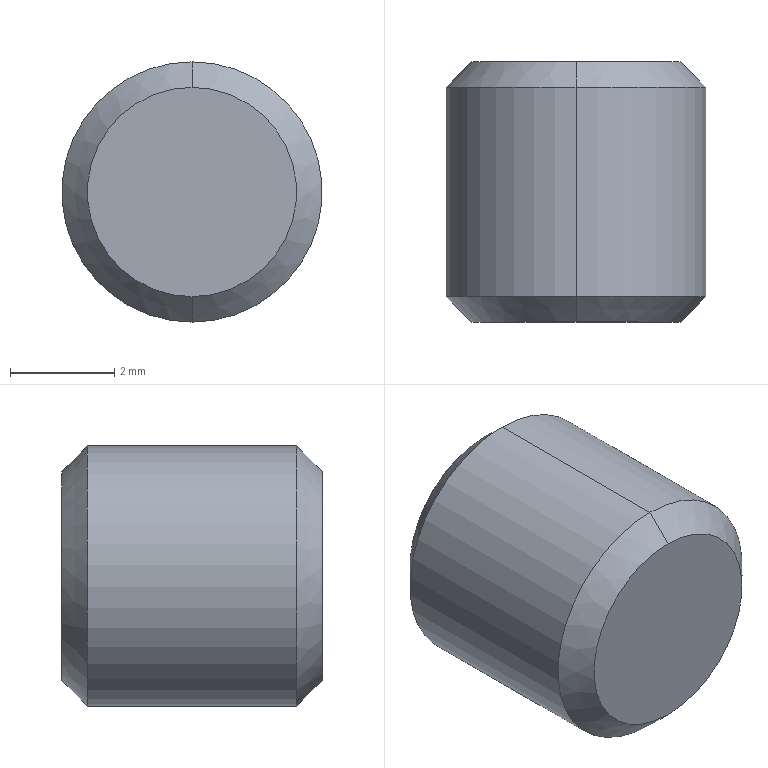Part | STEP file | 2-2 | 1 solid | 15 faces | box 5 x 5 x 5 mm | volume 86.524 mm3 | plane 9 | cone 4 | cylinder 2 | commonest cylinder face diameters 5 x2
STEP:
#1=CARTESIAN_POINT('',(0.,0.,0.));
#2=DIRECTION('',(0.,0.,1.));
#3=DIRECTION('',(1.,0.,0.));
#4=AXIS2_PLACEMENT_3D('',#1,#2,#3);
#5=CARTESIAN_POINT('',(10.278,45.,1.25));
#6=VERTEX_POINT('',#5);
#7=CARTESIAN_POINT('',(11.722,45.,1.25));
#8=VERTEX_POINT('',#7);
#9=CARTESIAN_POINT('',(10.278,45.,1.25));
#10=DIRECTION('',(1.,0.,0.));
#11=VECTOR('',#10,1.);
#12=LINE('',#9,#11);
#13=CARTESIAN_POINT('',(11.,45.,0.));
#14=DIRECTION('',(0.,1.,0.));
#15=DIRECTION('',(0.,0.,-1.));
#16=AXIS2_PLACEMENT_3D('',#13,#14,#15);
#17=PLANE('',#16);
#18=CARTESIAN_POINT('',(-1.25,0.7217));
#19=DIRECTION('',(0.,-1.));
#20=VECTOR('',#19,1.);
#21=LINE('',#18,#20);
#22=(GEOMETRIC_REPRESENTATION_CONTEXT(2)PARAMETRIC_REPRESENTATION_CONTEXT()REPRESENTATION_CONTEXT('',''));
#23=DEFINITIONAL_REPRESENTATION('',(#21),#22);
#24=PCURVE('',#17,#23);
#25=CARTESIAN_POINT('',(10.278,46.5,1.25));
#26=DIRECTION('',(0.,0.,1.));
#27=DIRECTION('',(1.,0.,0.));
#28=AXIS2_PLACEMENT_3D('',#25,#26,#27);
#29=PLANE('',#28);
#30=CARTESIAN_POINT('',(0.,-1.5));
#31=DIRECTION('',(1.,0.));
#32=VECTOR('',#31,1.);
#33=LINE('',#30,#32);
#34=(GEOMETRIC_REPRESENTATION_CONTEXT(2)PARAMETRIC_REPRESENTATION_CONTEXT()REPRESENTATION_CONTEXT('',''));
#35=DEFINITIONAL_REPRESENTATION('',(#33),#34);
#36=PCURVE('',#29,#35);
#37=SURFACE_CURVE('',#12,(#24,#36),.PCURVE_S1.);
#38=EDGE_CURVE('',#6,#8,#37,.T.);
#39=ORIENTED_EDGE('',*,*,#38,.T.);
#40=CARTESIAN_POINT('',(12.443,45.,0.));
#41=VERTEX_POINT('',#40);
#42=CARTESIAN_POINT('',(11.722,45.,1.25));
#43=DIRECTION('',(0.5,0.,-0.866));
#44=VECTOR('',#43,1.);
#45=LINE('',#42,#44);
#46=CARTESIAN_POINT('',(-1.25,-0.7217));
#47=DIRECTION('',(0.866,-0.5));
#48=VECTOR('',#47,1.);
#49=LINE('',#46,#48);
#50=(GEOMETRIC_REPRESENTATION_CONTEXT(2)PARAMETRIC_REPRESENTATION_CONTEXT()REPRESENTATION_CONTEXT('',''));
#51=DEFINITIONAL_REPRESENTATION('',(#49),#50);
#52=PCURVE('',#17,#51);
#53=CARTESIAN_POINT('',(11.722,46.5,1.25));
#54=DIRECTION('',(0.866,0.,0.5));
#55=DIRECTION('',(0.,-1.,0.));
#56=AXIS2_PLACEMENT_3D('',#53,#54,#55);
#57=PLANE('',#56);
#58=CARTESIAN_POINT('',(1.5,0.));
#59=DIRECTION('',(0.,1.));
#60=VECTOR('',#59,1.);
#61=LINE('',#58,#60);
#62=(GEOMETRIC_REPRESENTATION_CONTEXT(2)PARAMETRIC_REPRESENTATION_CONTEXT()REPRESENTATION_CONTEXT('',''));
#63=DEFINITIONAL_REPRESENTATION('',(#61),#62);
#64=PCURVE('',#57,#63);
#65=SURFACE_CURVE('',#45,(#52,#64),.PCURVE_S1.);
#66=EDGE_CURVE('',#8,#41,#65,.T.);
#67=ORIENTED_EDGE('',*,*,#66,.T.);
#68=CARTESIAN_POINT('',(11.722,45.,-1.25));
#69=VERTEX_POINT('',#68);
#70=CARTESIAN_POINT('',(12.443,45.,0.));
#71=DIRECTION('',(-0.5,0.,-0.866));
#72=VECTOR('',#71,1.);
#73=LINE('',#70,#72);
#74=CARTESIAN_POINT('',(0.,-1.443));
#75=DIRECTION('',(0.866,0.5));
#76=VECTOR('',#75,1.);
#77=LINE('',#74,#76);
#78=(GEOMETRIC_REPRESENTATION_CONTEXT(2)PARAMETRIC_REPRESENTATION_CONTEXT()REPRESENTATION_CONTEXT('',''));
#79=DEFINITIONAL_REPRESENTATION('',(#77),#78);
#80=PCURVE('',#17,#79);
#81=CARTESIAN_POINT('',(12.443,46.5,0.));
#82=DIRECTION('',(0.866,0.,-0.5));
#83=DIRECTION('',(0.,-1.,0.));
#84=AXIS2_PLACEMENT_3D('',#81,#82,#83);
#85=PLANE('',#84);
#86=CARTESIAN_POINT('',(1.5,0.));
#87=DIRECTION('',(0.,1.));
#88=VECTOR('',#87,1.);
#89=LINE('',#86,#88);
#90=(GEOMETRIC_REPRESENTATION_CONTEXT(2)PARAMETRIC_REPRESENTATION_CONTEXT()REPRESENTATION_CONTEXT('',''));
#91=DEFINITIONAL_REPRESENTATION('',(#89),#90);
#92=PCURVE('',#85,#91);
#93=SURFACE_CURVE('',#73,(#80,#92),.PCURVE_S1.);
#94=EDGE_CURVE('',#41,#69,#93,.T.);
#95=ORIENTED_EDGE('',*,*,#94,.T.);
#96=CARTESIAN_POINT('',(10.278,45.,-1.25));
#97=VERTEX_POINT('',#96);
#98=CARTESIAN_POINT('',(11.722,45.,-1.25));
#99=DIRECTION('',(-1.,0.,0.));
#100=VECTOR('',#99,1.);
#101=LINE('',#98,#100);
#102=CARTESIAN_POINT('',(1.25,-0.7217));
#103=DIRECTION('',(0.,1.));
#104=VECTOR('',#103,1.);
#105=LINE('',#102,#104);
#106=(GEOMETRIC_REPRESENTATION_CONTEXT(2)PARAMETRIC_REPRESENTATION_CONTEXT()REPRESENTATION_CONTEXT('',''));
#107=DEFINITIONAL_REPRESENTATION('',(#105),#106);
#108=PCURVE('',#17,#107);
#109=CARTESIAN_POINT('',(11.722,46.5,-1.25));
#110=DIRECTION('',(0.,0.,-1.));
#111=DIRECTION('',(-1.,0.,0.));
#112=AXIS2_PLACEMENT_3D('',#109,#110,#111);
#113=PLANE('',#112);
#114=CARTESIAN_POINT('',(0.,-1.5));
#115=DIRECTION('',(1.,0.));
#116=VECTOR('',#115,1.);
#117=LINE('',#114,#116);
#118=(GEOMETRIC_REPRESENTATION_CONTEXT(2)PARAMETRIC_REPRESENTATION_CONTEXT()REPRESENTATION_CONTEXT('',''));
#119=DEFINITIONAL_REPRESENTATION('',(#117),#118);
#120=PCURVE('',#113,#119);
#121=SURFACE_CURVE('',#101,(#108,#120),.PCURVE_S1.);
#122=EDGE_CURVE('',#69,#97,#121,.T.);
#123=ORIENTED_EDGE('',*,*,#122,.T.);
#124=CARTESIAN_POINT('',(9.557,45.,0.));
#125=VERTEX_POINT('',#124);
#126=CARTESIAN_POINT('',(10.278,45.,-1.25));
#127=DIRECTION('',(-0.5,0.,0.866));
#128=VECTOR('',#127,1.);
#129=LINE('',#126,#128);
#130=CARTESIAN_POINT('',(1.25,0.7217));
#131=DIRECTION('',(-0.866,0.5));
#132=VECTOR('',#131,1.);
#133=LINE('',#130,#132);
#134=(GEOMETRIC_REPRESENTATION_CONTEXT(2)PARAMETRIC_REPRESENTATION_CONTEXT()REPRESENTATION_CONTEXT('',''));
#135=DEFINITIONAL_REPRESENTATION('',(#133),#134);
#136=PCURVE('',#17,#135);
#137=CARTESIAN_POINT('',(10.278,46.5,-1.25));
#138=DIRECTION('',(-0.866,0.,-0.5));
#139=DIRECTION('',(-0.5,0.,0.866));
#140=AXIS2_PLACEMENT_3D('',#137,#138,#139);
#141=PLANE('',#140);
#142=CARTESIAN_POINT('',(0.,-1.5));
#143=DIRECTION('',(1.,0.));
#144=VECTOR('',#143,1.);
#145=LINE('',#142,#144);
#146=(GEOMETRIC_REPRESENTATION_CONTEXT(2)PARAMETRIC_REPRESENTATION_CONTEXT()REPRESENTATION_CONTEXT('',''));
#147=DEFINITIONAL_REPRESENTATION('',(#145),#146);
#148=PCURVE('',#141,#147);
#149=SURFACE_CURVE('',#129,(#136,#148),.PCURVE_S1.);
#150=EDGE_CURVE('',#97,#125,#149,.T.);
#151=ORIENTED_EDGE('',*,*,#150,.T.);
#152=CARTESIAN_POINT('',(9.557,45.,0.));
#153=DIRECTION('',(0.5,0.,0.866));
#154=VECTOR('',#153,1.);
#155=LINE('',#152,#154);
#156=CARTESIAN_POINT('',(0.,1.443));
#157=DIRECTION('',(-0.866,-0.5));
#158=VECTOR('',#157,1.);
#159=LINE('',#156,#158);
#160=(GEOMETRIC_REPRESENTATION_CONTEXT(2)PARAMETRIC_REPRESENTATION_CONTEXT()REPRESENTATION_CONTEXT('',''));
#161=DEFINITIONAL_REPRESENTATION('',(#159),#160);
#162=PCURVE('',#17,#161);
#163=CARTESIAN_POINT('',(9.557,46.5,0.));
#164=DIRECTION('',(-0.866,0.,0.5));
#165=DIRECTION('',(0.,1.,0.));
#166=AXIS2_PLACEMENT_3D('',#163,#164,#165);
#167=PLANE('',#166);
#168=CARTESIAN_POINT('',(-1.5,0.));
#169=DIRECTION('',(0.,-1.));
#170=VECTOR('',#169,1.);
#171=LINE('',#168,#170);
#172=(GEOMETRIC_REPRESENTATION_CONTEXT(2)PARAMETRIC_REPRESENTATION_CONTEXT()REPRESENTATION_CONTEXT('',''));
#173=DEFINITIONAL_REPRESENTATION('',(#171),#172);
#174=PCURVE('',#167,#173);
#175=SURFACE_CURVE('',#155,(#162,#174),.PCURVE_S1.);
#176=EDGE_CURVE('',#125,#6,#175,.T.);
#177=ORIENTED_EDGE('',*,*,#176,.T.);
#178=EDGE_LOOP('',(#39,#67,#95,#123,#151,#177));
#179=FACE_BOUND('',#178,.T.);
#180=ADVANCED_FACE('',(#179),#17,.T.);
#181=CARTESIAN_POINT('',(12.443,46.5,0.));
#182=VERTEX_POINT('',#181);
#183=CARTESIAN_POINT('',(12.443,46.5,0.));
#184=DIRECTION('',(0.,1.,0.));
#185=VECTOR('',#184,1.);
#186=LINE('',#183,#185);
#187=CARTESIAN_POINT('',(0.,0.));
#188=DIRECTION('',(-1.,0.));
#189=VECTOR('',#188,1.);
#190=LINE('',#187,#189);
#191=(GEOMETRIC_REPRESENTATION_CONTEXT(2)PARAMETRIC_REPRESENTATION_CONTEXT()REPRESENTATION_CONTEXT('',''));
#192=DEFINITIONAL_REPRESENTATION('',(#190),#191);
#193=PCURVE('',#85,#192);
#194=CARTESIAN_POINT('',(0.,1.443));
#195=DIRECTION('',(-1.,0.));
#196=VECTOR('',#195,1.);
#197=LINE('',#194,#196);
#198=(GEOMETRIC_REPRESENTATION_CONTEXT(2)PARAMETRIC_REPRESENTATION_CONTEXT()REPRESENTATION_CONTEXT('',''));
#199=DEFINITIONAL_REPRESENTATION('',(#197),#198);
#200=PCURVE('',#57,#199);
#201=SURFACE_CURVE('',#186,(#193,#200),.PCURVE_S1.);
#202=EDGE_CURVE('',#41,#182,#201,.T.);
#203=ORIENTED_EDGE('',*,*,#202,.T.);
#204=CARTESIAN_POINT('',(11.722,46.5,-1.25));
#205=VERTEX_POINT('',#204);
#206=CARTESIAN_POINT('',(11.722,46.5,-1.25));
#207=DIRECTION('',(0.5,0.,0.866));
#208=VECTOR('',#207,1.);
#209=LINE('',#206,#208);
#210=CARTESIAN_POINT('',(0.,1.443));
#211=DIRECTION('',(0.,-1.));
#212=VECTOR('',#211,1.);
#213=LINE('',#210,#212);
#214=(GEOMETRIC_REPRESENTATION_CONTEXT(2)PARAMETRIC_REPRESENTATION_CONTEXT()REPRESENTATION_CONTEXT('',''));
#215=DEFINITIONAL_REPRESENTATION('',(#213),#214);
#216=PCURVE('',#85,#215);
#217=CARTESIAN_POINT('',(11.,46.5,-1.005));
#218=DIRECTION('',(0.,1.,0.));
#219=DIRECTION('',(0.,0.,-1.));
#220=AXIS2_PLACEMENT_3D('',#217,#218,#219);
#221=PLANE('',#220);
#222=CARTESIAN_POINT('',(0.2452,-0.7217));
#223=DIRECTION('',(-0.866,-0.5));
#224=VECTOR('',#223,1.);
#225=LINE('',#222,#224);
#226=(GEOMETRIC_REPRESENTATION_CONTEXT(2)PARAMETRIC_REPRESENTATION_CONTEXT()REPRESENTATION_CONTEXT('',''));
#227=DEFINITIONAL_REPRESENTATION('',(#225),#226);
#228=PCURVE('',#221,#227);
#229=SURFACE_CURVE('',#209,(#216,#228),.PCURVE_S1.);
#230=EDGE_CURVE('',#205,#182,#229,.T.);
#231=ORIENTED_EDGE('',*,*,#230,.F.);
#232=CARTESIAN_POINT('',(11.722,46.5,-1.25));
#233=DIRECTION('',(0.,-1.,0.));
#234=VECTOR('',#233,1.);
#235=LINE('',#232,#234);
#236=CARTESIAN_POINT('',(0.,1.443));
#237=DIRECTION('',(1.,0.));
#238=VECTOR('',#237,1.);
#239=LINE('',#236,#238);
#240=(GEOMETRIC_REPRESENTATION_CONTEXT(2)PARAMETRIC_REPRESENTATION_CONTEXT()REPRESENTATION_CONTEXT('',''));
#241=DEFINITIONAL_REPRESENTATION('',(#239),#240);
#242=PCURVE('',#85,#241);
#243=CARTESIAN_POINT('',(0.,0.));
#244=DIRECTION('',(0.,-1.));
#245=VECTOR('',#244,1.);
#246=LINE('',#243,#245);
#247=(GEOMETRIC_REPRESENTATION_CONTEXT(2)PARAMETRIC_REPRESENTATION_CONTEXT()REPRESENTATION_CONTEXT('',''));
#248=DEFINITIONAL_REPRESENTATION('',(#246),#247);
#249=PCURVE('',#113,#248);
#250=SURFACE_CURVE('',#235,(#242,#249),.PCURVE_S1.);
#251=EDGE_CURVE('',#205,#69,#250,.T.);
#252=ORIENTED_EDGE('',*,*,#251,.T.);
#253=ORIENTED_EDGE('',*,*,#94,.F.);
#254=EDGE_LOOP('',(#203,#231,#252,#253));
#255=FACE_BOUND('',#254,.T.);
#256=ADVANCED_FACE('',(#255),#85,.F.);
#257=CARTESIAN_POINT('',(11.722,46.5,1.25));
#258=VERTEX_POINT('',#257);
#259=CARTESIAN_POINT('',(11.722,46.5,1.25));
#260=DIRECTION('',(0.,1.,0.));
#261=VECTOR('',#260,1.);
#262=LINE('',#259,#261);
#263=CARTESIAN_POINT('',(0.,0.));
#264=DIRECTION('',(-1.,0.));
#265=VECTOR('',#264,1.);
#266=LINE('',#263,#265);
#267=(GEOMETRIC_REPRESENTATION_CONTEXT(2)PARAMETRIC_REPRESENTATION_CONTEXT()REPRESENTATION_CONTEXT('',''));
#268=DEFINITIONAL_REPRESENTATION('',(#266),#267);
#269=PCURVE('',#57,#268);
#270=CARTESIAN_POINT('',(1.443,0.));
#271=DIRECTION('',(0.,1.));
#272=VECTOR('',#271,1.);
#273=LINE('',#270,#272);
#274=(GEOMETRIC_REPRESENTATION_CONTEXT(2)PARAMETRIC_REPRESENTATION_CONTEXT()REPRESENTATION_CONTEXT('',''));
#275=DEFINITIONAL_REPRESENTATION('',(#273),#274);
#276=PCURVE('',#29,#275);
#277=SURFACE_CURVE('',#262,(#269,#276),.PCURVE_S1.);
#278=EDGE_CURVE('',#8,#258,#277,.T.);
#279=ORIENTED_EDGE('',*,*,#278,.T.);
#280=CARTESIAN_POINT('',(12.443,46.5,0.));
#281=DIRECTION('',(-0.5,0.,0.866));
#282=VECTOR('',#281,1.);
#283=LINE('',#280,#282);
#284=CARTESIAN_POINT('',(0.,1.443));
#285=DIRECTION('',(0.,-1.));
#286=VECTOR('',#285,1.);
#287=LINE('',#284,#286);
#288=(GEOMETRIC_REPRESENTATION_CONTEXT(2)PARAMETRIC_REPRESENTATION_CONTEXT()REPRESENTATION_CONTEXT('',''));
#289=DEFINITIONAL_REPRESENTATION('',(#287),#288);
#290=PCURVE('',#57,#289);
#291=CARTESIAN_POINT('',(-1.005,-1.443));
#292=DIRECTION('',(-0.866,0.5));
#293=VECTOR('',#292,1.);
#294=LINE('',#291,#293);
#295=(GEOMETRIC_REPRESENTATION_CONTEXT(2)PARAMETRIC_REPRESENTATION_CONTEXT()REPRESENTATION_CONTEXT('',''));
#296=DEFINITIONAL_REPRESENTATION('',(#294),#295);
#297=PCURVE('',#221,#296);
#298=SURFACE_CURVE('',#283,(#290,#297),.PCURVE_S1.);
#299=EDGE_CURVE('',#182,#258,#298,.T.);
#300=ORIENTED_EDGE('',*,*,#299,.F.);
#301=ORIENTED_EDGE('',*,*,#202,.F.);
#302=ORIENTED_EDGE('',*,*,#66,.F.);
#303=EDGE_LOOP('',(#279,#300,#301,#302));
#304=FACE_BOUND('',#303,.T.);
#305=ADVANCED_FACE('',(#304),#57,.F.);
#306=CARTESIAN_POINT('',(10.278,46.5,1.25));
#307=VERTEX_POINT('',#306);
#308=CARTESIAN_POINT('',(10.278,46.5,1.25));
#309=DIRECTION('',(0.,1.,0.));
#310=VECTOR('',#309,1.);
#311=LINE('',#308,#310);
#312=CARTESIAN_POINT('',(0.,0.));
#313=DIRECTION('',(0.,1.));
#314=VECTOR('',#313,1.);
#315=LINE('',#312,#314);
#316=(GEOMETRIC_REPRESENTATION_CONTEXT(2)PARAMETRIC_REPRESENTATION_CONTEXT()REPRESENTATION_CONTEXT('',''));
#317=DEFINITIONAL_REPRESENTATION('',(#315),#316);
#318=PCURVE('',#29,#317);
#319=CARTESIAN_POINT('',(0.,-1.443));
#320=DIRECTION('',(1.,0.));
#321=VECTOR('',#320,1.);
#322=LINE('',#319,#321);
#323=(GEOMETRIC_REPRESENTATION_CONTEXT(2)PARAMETRIC_REPRESENTATION_CONTEXT()REPRESENTATION_CONTEXT('',''));
#324=DEFINITIONAL_REPRESENTATION('',(#322),#323);
#325=PCURVE('',#167,#324);
#326=SURFACE_CURVE('',#311,(#318,#325),.PCURVE_S1.);
#327=EDGE_CURVE('',#6,#307,#326,.T.);
#328=ORIENTED_EDGE('',*,*,#327,.T.);
#329=CARTESIAN_POINT('',(11.,46.5,1.25));
#330=DIRECTION('',(-1.,0.,0.));
#331=VECTOR('',#330,1.);
#332=LINE('',#329,#331);
#333=CARTESIAN_POINT('',(0.7217,0.));
#334=DIRECTION('',(-1.,0.));
#335=VECTOR('',#334,1.);
#336=LINE('',#333,#335);
#337=(GEOMETRIC_REPRESENTATION_CONTEXT(2)PARAMETRIC_REPRESENTATION_CONTEXT()REPRESENTATION_CONTEXT('',''));
#338=DEFINITIONAL_REPRESENTATION('',(#336),#337);
#339=PCURVE('',#29,#338);
#340=CARTESIAN_POINT('',(-2.255,0.));
#341=DIRECTION('',(0.,1.));
#342=VECTOR('',#341,1.);
#343=LINE('',#340,#342);
#344=(GEOMETRIC_REPRESENTATION_CONTEXT(2)PARAMETRIC_REPRESENTATION_CONTEXT()REPRESENTATION_CONTEXT('',''));
#345=DEFINITIONAL_REPRESENTATION('',(#343),#344);
#346=PCURVE('',#221,#345);
#347=SURFACE_CURVE('',#332,(#339,#346),.PCURVE_S1.);
#348=EDGE_CURVE('',#258,#307,#347,.T.);
#349=ORIENTED_EDGE('',*,*,#348,.F.);
#350=ORIENTED_EDGE('',*,*,#278,.F.);
#351=ORIENTED_EDGE('',*,*,#38,.F.);
#352=EDGE_LOOP('',(#328,#349,#350,#351));
#353=FACE_BOUND('',#352,.T.);
#354=ADVANCED_FACE('',(#353),#29,.F.);
#355=CARTESIAN_POINT('',(9.557,46.5,0.));
#356=VERTEX_POINT('',#355);
#357=CARTESIAN_POINT('',(9.557,46.5,0.));
#358=DIRECTION('',(0.,1.,0.));
#359=VECTOR('',#358,1.);
#360=LINE('',#357,#359);
#361=CARTESIAN_POINT('',(0.,0.));
#362=DIRECTION('',(1.,0.));
#363=VECTOR('',#362,1.);
#364=LINE('',#361,#363);
#365=(GEOMETRIC_REPRESENTATION_CONTEXT(2)PARAMETRIC_REPRESENTATION_CONTEXT()REPRESENTATION_CONTEXT('',''));
#366=DEFINITIONAL_REPRESENTATION('',(#364),#365);
#367=PCURVE('',#167,#366);
#368=CARTESIAN_POINT('',(1.443,0.));
#369=DIRECTION('',(0.,1.));
#370=VECTOR('',#369,1.);
#371=LINE('',#368,#370);
#372=(GEOMETRIC_REPRESENTATION_CONTEXT(2)PARAMETRIC_REPRESENTATION_CONTEXT()REPRESENTATION_CONTEXT('',''));
#373=DEFINITIONAL_REPRESENTATION('',(#371),#372);
#374=PCURVE('',#141,#373);
#375=SURFACE_CURVE('',#360,(#367,#374),.PCURVE_S1.);
#376=EDGE_CURVE('',#125,#356,#375,.T.);
#377=ORIENTED_EDGE('',*,*,#376,.T.);
#378=CARTESIAN_POINT('',(10.278,46.5,1.25));
#379=DIRECTION('',(-0.5,0.,-0.866));
#380=VECTOR('',#379,1.);
#381=LINE('',#378,#380);
#382=CARTESIAN_POINT('',(0.,-1.443));
#383=DIRECTION('',(0.,1.));
#384=VECTOR('',#383,1.);
#385=LINE('',#382,#384);
#386=(GEOMETRIC_REPRESENTATION_CONTEXT(2)PARAMETRIC_REPRESENTATION_CONTEXT()REPRESENTATION_CONTEXT('',''));
#387=DEFINITIONAL_REPRESENTATION('',(#385),#386);
#388=PCURVE('',#167,#387);
#389=CARTESIAN_POINT('',(-2.255,0.7217));
#390=DIRECTION('',(0.866,0.5));
#391=VECTOR('',#390,1.);
#392=LINE('',#389,#391);
#393=(GEOMETRIC_REPRESENTATION_CONTEXT(2)PARAMETRIC_REPRESENTATION_CONTEXT()REPRESENTATION_CONTEXT('',''));
#394=DEFINITIONAL_REPRESENTATION('',(#392),#393);
#395=PCURVE('',#221,#394);
#396=SURFACE_CURVE('',#381,(#388,#395),.PCURVE_S1.);
#397=EDGE_CURVE('',#307,#356,#396,.T.);
#398=ORIENTED_EDGE('',*,*,#397,.F.);
#399=ORIENTED_EDGE('',*,*,#327,.F.);
#400=ORIENTED_EDGE('',*,*,#176,.F.);
#401=EDGE_LOOP('',(#377,#398,#399,#400));
#402=FACE_BOUND('',#401,.T.);
#403=ADVANCED_FACE('',(#402),#167,.F.);
#404=CARTESIAN_POINT('',(10.278,46.5,-1.25));
#405=VERTEX_POINT('',#404);
#406=CARTESIAN_POINT('',(10.278,46.5,-1.25));
#407=DIRECTION('',(0.,1.,0.));
#408=VECTOR('',#407,1.);
#409=LINE('',#406,#408);
#410=CARTESIAN_POINT('',(0.,0.));
#411=DIRECTION('',(0.,1.));
#412=VECTOR('',#411,1.);
#413=LINE('',#410,#412);
#414=(GEOMETRIC_REPRESENTATION_CONTEXT(2)PARAMETRIC_REPRESENTATION_CONTEXT()REPRESENTATION_CONTEXT('',''));
#415=DEFINITIONAL_REPRESENTATION('',(#413),#414);
#416=PCURVE('',#141,#415);
#417=CARTESIAN_POINT('',(1.443,0.));
#418=DIRECTION('',(0.,1.));
#419=VECTOR('',#418,1.);
#420=LINE('',#417,#419);
#421=(GEOMETRIC_REPRESENTATION_CONTEXT(2)PARAMETRIC_REPRESENTATION_CONTEXT()REPRESENTATION_CONTEXT('',''));
#422=DEFINITIONAL_REPRESENTATION('',(#420),#421);
#423=PCURVE('',#113,#422);
#424=SURFACE_CURVE('',#409,(#416,#423),.PCURVE_S1.);
#425=EDGE_CURVE('',#97,#405,#424,.T.);
#426=ORIENTED_EDGE('',*,*,#425,.T.);
#427=CARTESIAN_POINT('',(9.557,46.5,0.));
#428=DIRECTION('',(0.5,0.,-0.866));
#429=VECTOR('',#428,1.);
#430=LINE('',#427,#429);
#431=CARTESIAN_POINT('',(1.443,0.));
#432=DIRECTION('',(-1.,0.));
#433=VECTOR('',#432,1.);
#434=LINE('',#431,#433);
#435=(GEOMETRIC_REPRESENTATION_CONTEXT(2)PARAMETRIC_REPRESENTATION_CONTEXT()REPRESENTATION_CONTEXT('',''));
#436=DEFINITIONAL_REPRESENTATION('',(#434),#435);
#437=PCURVE('',#141,#436);
#438=CARTESIAN_POINT('',(-1.005,1.443));
#439=DIRECTION('',(0.866,-0.5));
#440=VECTOR('',#439,1.);
#441=LINE('',#438,#440);
#442=(GEOMETRIC_REPRESENTATION_CONTEXT(2)PARAMETRIC_REPRESENTATION_CONTEXT()REPRESENTATION_CONTEXT('',''));
#443=DEFINITIONAL_REPRESENTATION('',(#441),#442);
#444=PCURVE('',#221,#443);
#445=SURFACE_CURVE('',#430,(#437,#444),.PCURVE_S1.);
#446=EDGE_CURVE('',#356,#405,#445,.T.);
#447=ORIENTED_EDGE('',*,*,#446,.F.);
#448=ORIENTED_EDGE('',*,*,#376,.F.);
#449=ORIENTED_EDGE('',*,*,#150,.F.);
#450=EDGE_LOOP('',(#426,#447,#448,#449));
#451=FACE_BOUND('',#450,.T.);
#452=ADVANCED_FACE('',(#451),#141,.F.);
#453=ORIENTED_EDGE('',*,*,#251,.F.);
#454=CARTESIAN_POINT('',(11.,46.5,-1.25));
#455=DIRECTION('',(1.,0.,0.));
#456=VECTOR('',#455,1.);
#457=LINE('',#454,#456);
#458=CARTESIAN_POINT('',(0.7217,0.));
#459=DIRECTION('',(-1.,0.));
#460=VECTOR('',#459,1.);
#461=LINE('',#458,#460);
#462=(GEOMETRIC_REPRESENTATION_CONTEXT(2)PARAMETRIC_REPRESENTATION_CONTEXT()REPRESENTATION_CONTEXT('',''));
#463=DEFINITIONAL_REPRESENTATION('',(#461),#462);
#464=PCURVE('',#113,#463);
#465=CARTESIAN_POINT('',(0.2452,0.));
#466=DIRECTION('',(0.,-1.));
#467=VECTOR('',#466,1.);
#468=LINE('',#465,#467);
#469=(GEOMETRIC_REPRESENTATION_CONTEXT(2)PARAMETRIC_REPRESENTATION_CONTEXT()REPRESENTATION_CONTEXT('',''));
#470=DEFINITIONAL_REPRESENTATION('',(#468),#469);
#471=PCURVE('',#221,#470);
#472=SURFACE_CURVE('',#457,(#464,#471),.PCURVE_S1.);
#473=EDGE_CURVE('',#405,#205,#472,.T.);
#474=ORIENTED_EDGE('',*,*,#473,.F.);
#475=ORIENTED_EDGE('',*,*,#425,.F.);
#476=ORIENTED_EDGE('',*,*,#122,.F.);
#477=EDGE_LOOP('',(#453,#474,#475,#476));
#478=FACE_BOUND('',#477,.T.);
#479=ADVANCED_FACE('',(#478),#113,.F.);
#480=ORIENTED_EDGE('',*,*,#446,.T.);
#481=ORIENTED_EDGE('',*,*,#473,.T.);
#482=ORIENTED_EDGE('',*,*,#230,.T.);
#483=ORIENTED_EDGE('',*,*,#299,.T.);
#484=ORIENTED_EDGE('',*,*,#348,.T.);
#485=ORIENTED_EDGE('',*,*,#397,.T.);
#486=EDGE_LOOP('',(#480,#481,#482,#483,#484,#485));
#487=FACE_BOUND('',#486,.T.);
#488=CARTESIAN_POINT('',(11.,46.5,-2.01));
#489=VERTEX_POINT('',#488);
#490=CARTESIAN_POINT('',(11.,46.5,2.01));
#491=VERTEX_POINT('',#490);
#492=CARTESIAN_POINT('',(11.,46.5,0.));
#493=DIRECTION('',(0.,-1.,0.));
#494=DIRECTION('',(0.,0.,-1.));
#495=AXIS2_PLACEMENT_3D('',#492,#493,#494);
#496=CIRCLE('',#495,2.01);
#497=CARTESIAN_POINT('',(1.005,0.));
#498=CARTESIAN_POINT('',(1.005,-3.481));
#499=CARTESIAN_POINT('',(-2.01,-1.74));
#500=CARTESIAN_POINT('',(-5.024,0.));
#501=CARTESIAN_POINT('',(-2.01,1.74));
#502=CARTESIAN_POINT('',(1.005,3.481));
#503=CARTESIAN_POINT('',(1.005,0.));
#504=(BOUNDED_CURVE()B_SPLINE_CURVE(2,(#497,#498,#499,#500,#501,#502,#503),.UNSPECIFIED.,.T.,.F.)B_SPLINE_CURVE_WITH_KNOTS((1,2,2,2,2,1),(-2.094,0.,2.094,4.189,6.283,8.378),.UNSPECIFIED.)CURVE()GEOMETRIC_REPRESENTATION_ITEM()RATIONAL_B_SPLINE_CURVE((1.,0.5,1.,0.5,1.,0.5,1.))REPRESENTATION_ITEM(''));
#505=(GEOMETRIC_REPRESENTATION_CONTEXT(2)PARAMETRIC_REPRESENTATION_CONTEXT()REPRESENTATION_CONTEXT('',''));
#506=DEFINITIONAL_REPRESENTATION('',(#504),#505);
#507=PCURVE('',#221,#506);
#508=CARTESIAN_POINT('',(11.,46.01,0.));
#509=DIRECTION('',(0.,-1.,0.));
#510=DIRECTION('',(0.,0.,-1.));
#511=AXIS2_PLACEMENT_3D('',#508,#509,#510);
#512=CONICAL_SURFACE('',#511,2.5,0.7854);
#513=CARTESIAN_POINT('',(0.,-0.4905));
#514=DIRECTION('',(1.,0.));
#515=VECTOR('',#514,1.);
#516=LINE('',#513,#515);
#517=(GEOMETRIC_REPRESENTATION_CONTEXT(2)PARAMETRIC_REPRESENTATION_CONTEXT()REPRESENTATION_CONTEXT('',''));
#518=DEFINITIONAL_REPRESENTATION('',(#516),#517);
#519=PCURVE('',#512,#518);
#520=SURFACE_CURVE('',#496,(#507,#519),.PCURVE_S1.);
#521=EDGE_CURVE('',#489,#491,#520,.T.);
#522=ORIENTED_EDGE('',*,*,#521,.F.);
#523=CARTESIAN_POINT('',(11.,46.5,0.));
#524=DIRECTION('',(0.,-1.,0.));
#525=DIRECTION('',(0.,0.,-1.));
#526=AXIS2_PLACEMENT_3D('',#523,#524,#525);
#527=CIRCLE('',#526,2.01);
#528=CARTESIAN_POINT('',(1.005,0.));
#529=CARTESIAN_POINT('',(1.005,-3.481));
#530=CARTESIAN_POINT('',(-2.01,-1.74));
#531=CARTESIAN_POINT('',(-5.024,0.));
#532=CARTESIAN_POINT('',(-2.01,1.74));
#533=CARTESIAN_POINT('',(1.005,3.481));
#534=CARTESIAN_POINT('',(1.005,0.));
#535=(BOUNDED_CURVE()B_SPLINE_CURVE(2,(#528,#529,#530,#531,#532,#533,#534),.UNSPECIFIED.,.T.,.F.)B_SPLINE_CURVE_WITH_KNOTS((1,2,2,2,2,1),(-2.094,0.,2.094,4.189,6.283,8.378),.UNSPECIFIED.)CURVE()GEOMETRIC_REPRESENTATION_ITEM()RATIONAL_B_SPLINE_CURVE((1.,0.5,1.,0.5,1.,0.5,1.))REPRESENTATION_ITEM(''));
#536=(GEOMETRIC_REPRESENTATION_CONTEXT(2)PARAMETRIC_REPRESENTATION_CONTEXT()REPRESENTATION_CONTEXT('',''));
#537=DEFINITIONAL_REPRESENTATION('',(#535),#536);
#538=PCURVE('',#221,#537);
#539=CARTESIAN_POINT('',(11.,46.01,0.));
#540=DIRECTION('',(0.,-1.,0.));
#541=DIRECTION('',(0.,0.,-1.));
#542=AXIS2_PLACEMENT_3D('',#539,#540,#541);
#543=CONICAL_SURFACE('',#542,2.5,0.7854);
#544=CARTESIAN_POINT('',(0.,-0.4905));
#545=DIRECTION('',(1.,0.));
#546=VECTOR('',#545,1.);
#547=LINE('',#544,#546);
#548=(GEOMETRIC_REPRESENTATION_CONTEXT(2)PARAMETRIC_REPRESENTATION_CONTEXT()REPRESENTATION_CONTEXT('',''));
#549=DEFINITIONAL_REPRESENTATION('',(#547),#548);
#550=PCURVE('',#543,#549);
#551=SURFACE_CURVE('',#527,(#538,#550),.PCURVE_S1.);
#552=EDGE_CURVE('',#491,#489,#551,.T.);
#553=ORIENTED_EDGE('',*,*,#552,.F.);
#554=EDGE_LOOP('',(#522,#553));
#555=FACE_BOUND('',#554,.T.);
#556=ADVANCED_FACE('',(#487,#555),#221,.T.);
#557=CARTESIAN_POINT('',(11.,41.5,2.009));
#558=VERTEX_POINT('',#557);
#559=CARTESIAN_POINT('',(11.,41.5,-2.009));
#560=VERTEX_POINT('',#559);
#561=CARTESIAN_POINT('',(11.,41.5,0.));
#562=DIRECTION('',(0.,1.,0.));
#563=DIRECTION('',(0.,0.,1.));
#564=AXIS2_PLACEMENT_3D('',#561,#562,#563);
#565=CIRCLE('',#564,2.009);
#566=CARTESIAN_POINT('',(11.,41.5,-1.005));
#567=DIRECTION('',(0.,-1.,0.));
#568=DIRECTION('',(0.,0.,-1.));
#569=AXIS2_PLACEMENT_3D('',#566,#567,#568);
#570=PLANE('',#569);
#571=CARTESIAN_POINT('',(-3.014,0.));
#572=CARTESIAN_POINT('',(-3.014,3.481));
#573=CARTESIAN_POINT('',(0.,1.74));
#574=CARTESIAN_POINT('',(3.014,0.));
#575=CARTESIAN_POINT('',(0.,-1.74));
#576=CARTESIAN_POINT('',(-3.014,-3.481));
#577=CARTESIAN_POINT('',(-3.014,0.));
#578=(BOUNDED_CURVE()B_SPLINE_CURVE(2,(#571,#572,#573,#574,#575,#576,#577),.UNSPECIFIED.,.T.,.F.)B_SPLINE_CURVE_WITH_KNOTS((1,2,2,2,2,1),(-2.094,0.,2.094,4.189,6.283,8.378),.UNSPECIFIED.)CURVE()GEOMETRIC_REPRESENTATION_ITEM()RATIONAL_B_SPLINE_CURVE((1.,0.5,1.,0.5,1.,0.5,1.))REPRESENTATION_ITEM(''));
#579=(GEOMETRIC_REPRESENTATION_CONTEXT(2)PARAMETRIC_REPRESENTATION_CONTEXT()REPRESENTATION_CONTEXT('',''));
#580=DEFINITIONAL_REPRESENTATION('',(#578),#579);
#581=PCURVE('',#570,#580);
#582=CARTESIAN_POINT('',(11.,41.99,0.));
#583=DIRECTION('',(0.,1.,0.));
#584=DIRECTION('',(0.,0.,1.));
#585=AXIS2_PLACEMENT_3D('',#582,#583,#584);
#586=CONICAL_SURFACE('',#585,2.5,0.7854);
#587=CARTESIAN_POINT('',(0.,-0.4905));
#588=DIRECTION('',(1.,0.));
#589=VECTOR('',#588,1.);
#590=LINE('',#587,#589);
#591=(GEOMETRIC_REPRESENTATION_CONTEXT(2)PARAMETRIC_REPRESENTATION_CONTEXT()REPRESENTATION_CONTEXT('',''));
#592=DEFINITIONAL_REPRESENTATION('',(#590),#591);
#593=PCURVE('',#586,#592);
#594=SURFACE_CURVE('',#565,(#581,#593),.PCURVE_S1.);
#595=EDGE_CURVE('',#558,#560,#594,.T.);
#596=ORIENTED_EDGE('',*,*,#595,.F.);
#597=CARTESIAN_POINT('',(11.,41.5,0.));
#598=DIRECTION('',(0.,1.,0.));
#599=DIRECTION('',(0.,0.,1.));
#600=AXIS2_PLACEMENT_3D('',#597,#598,#599);
#601=CIRCLE('',#600,2.009);
#602=CARTESIAN_POINT('',(-3.014,0.));
#603=CARTESIAN_POINT('',(-3.014,3.481));
#604=CARTESIAN_POINT('',(0.,1.74));
#605=CARTESIAN_POINT('',(3.014,0.));
#606=CARTESIAN_POINT('',(0.,-1.74));
#607=CARTESIAN_POINT('',(-3.014,-3.481));
#608=CARTESIAN_POINT('',(-3.014,0.));
#609=(BOUNDED_CURVE()B_SPLINE_CURVE(2,(#602,#603,#604,#605,#606,#607,#608),.UNSPECIFIED.,.T.,.F.)B_SPLINE_CURVE_WITH_KNOTS((1,2,2,2,2,1),(-2.094,0.,2.094,4.189,6.283,8.378),.UNSPECIFIED.)CURVE()GEOMETRIC_REPRESENTATION_ITEM()RATIONAL_B_SPLINE_CURVE((1.,0.5,1.,0.5,1.,0.5,1.))REPRESENTATION_ITEM(''));
#610=(GEOMETRIC_REPRESENTATION_CONTEXT(2)PARAMETRIC_REPRESENTATION_CONTEXT()REPRESENTATION_CONTEXT('',''));
#611=DEFINITIONAL_REPRESENTATION('',(#609),#610);
#612=PCURVE('',#570,#611);
#613=CARTESIAN_POINT('',(11.,41.99,0.));
#614=DIRECTION('',(0.,1.,0.));
#615=DIRECTION('',(0.,0.,1.));
#616=AXIS2_PLACEMENT_3D('',#613,#614,#615);
#617=CONICAL_SURFACE('',#616,2.5,0.7854);
#618=CARTESIAN_POINT('',(0.,-0.4905));
#619=DIRECTION('',(1.,0.));
#620=VECTOR('',#619,1.);
#621=LINE('',#618,#620);
#622=(GEOMETRIC_REPRESENTATION_CONTEXT(2)PARAMETRIC_REPRESENTATION_CONTEXT()REPRESENTATION_CONTEXT('',''));
#623=DEFINITIONAL_REPRESENTATION('',(#621),#622);
#624=PCURVE('',#617,#623);
#625=SURFACE_CURVE('',#601,(#612,#624),.PCURVE_S1.);
#626=EDGE_CURVE('',#560,#558,#625,.T.);
#627=ORIENTED_EDGE('',*,*,#626,.F.);
#628=EDGE_LOOP('',(#596,#627));
#629=FACE_BOUND('',#628,.T.);
#630=ADVANCED_FACE('',(#629),#570,.T.);
#631=CARTESIAN_POINT('',(11.,46.01,2.5));
#632=VERTEX_POINT('',#631);
#633=CARTESIAN_POINT('',(11.,46.01,2.5));
#634=DIRECTION('',(0.,-0.7071,0.7071));
#635=VECTOR('',#634,1.);
#636=LINE('',#633,#635);
#637=CARTESIAN_POINT('',(3.142,0.));
#638=DIRECTION('',(0.,1.));
#639=VECTOR('',#638,1.);
#640=LINE('',#637,#639);
#641=(GEOMETRIC_REPRESENTATION_CONTEXT(2)PARAMETRIC_REPRESENTATION_CONTEXT()REPRESENTATION_CONTEXT('',''));
#642=DEFINITIONAL_REPRESENTATION('',(#640),#641);
#643=PCURVE('',#543,#642);
#644=CARTESIAN_POINT('',(3.142,0.));
#645=DIRECTION('',(0.,1.));
#646=VECTOR('',#645,1.);
#647=LINE('',#644,#646);
#648=(GEOMETRIC_REPRESENTATION_CONTEXT(2)PARAMETRIC_REPRESENTATION_CONTEXT()REPRESENTATION_CONTEXT('',''));
#649=DEFINITIONAL_REPRESENTATION('',(#647),#648);
#650=PCURVE('',#512,#649);
#651=SURFACE_CURVE('',#636,(#643,#650),.PCURVE_S1.);
#652=EDGE_CURVE('',#491,#632,#651,.T.);
#653=ORIENTED_EDGE('',*,*,#652,.F.);
#654=ORIENTED_EDGE('',*,*,#552,.T.);
#655=CARTESIAN_POINT('',(11.,46.01,-2.5));
#656=VERTEX_POINT('',#655);
#657=CARTESIAN_POINT('',(11.,46.01,-2.5));
#658=DIRECTION('',(0.,-0.7071,-0.7071));
#659=VECTOR('',#658,1.);
#660=LINE('',#657,#659);
#661=CARTESIAN_POINT('',(6.283,0.));
#662=DIRECTION('',(0.,1.));
#663=VECTOR('',#662,1.);
#664=LINE('',#661,#663);
#665=(GEOMETRIC_REPRESENTATION_CONTEXT(2)PARAMETRIC_REPRESENTATION_CONTEXT()REPRESENTATION_CONTEXT('',''));
#666=DEFINITIONAL_REPRESENTATION('',(#664),#665);
#667=PCURVE('',#543,#666);
#668=CARTESIAN_POINT('',(0.,0.));
#669=DIRECTION('',(0.,1.));
#670=VECTOR('',#669,1.);
#671=LINE('',#668,#670);
#672=(GEOMETRIC_REPRESENTATION_CONTEXT(2)PARAMETRIC_REPRESENTATION_CONTEXT()REPRESENTATION_CONTEXT('',''));
#673=DEFINITIONAL_REPRESENTATION('',(#671),#672);
#674=PCURVE('',#512,#673);
#675=SURFACE_CURVE('',#660,(#667,#674),.PCURVE_S1.);
#676=EDGE_CURVE('',#489,#656,#675,.T.);
#677=ORIENTED_EDGE('',*,*,#676,.T.);
#678=CARTESIAN_POINT('',(11.,46.01,0.));
#679=DIRECTION('',(0.,-1.,0.));
#680=DIRECTION('',(0.,0.,1.));
#681=AXIS2_PLACEMENT_3D('',#678,#679,#680);
#682=CIRCLE('',#681,2.5);
#683=CARTESIAN_POINT('',(3.142,0.));
#684=DIRECTION('',(1.,0.));
#685=VECTOR('',#684,1.);
#686=LINE('',#683,#685);
#687=(GEOMETRIC_REPRESENTATION_CONTEXT(2)PARAMETRIC_REPRESENTATION_CONTEXT()REPRESENTATION_CONTEXT('',''));
#688=DEFINITIONAL_REPRESENTATION('',(#686),#687);
#689=PCURVE('',#543,#688);
#690=CARTESIAN_POINT('',(11.,44.,0.));
#691=DIRECTION('',(0.,1.,0.));
#692=DIRECTION('',(0.,0.,1.));
#693=AXIS2_PLACEMENT_3D('',#690,#691,#692);
#694=CYLINDRICAL_SURFACE('',#693,2.5);
#695=CARTESIAN_POINT('',(6.283,2.01));
#696=DIRECTION('',(-1.,0.));
#697=VECTOR('',#696,1.);
#698=LINE('',#695,#697);
#699=(GEOMETRIC_REPRESENTATION_CONTEXT(2)PARAMETRIC_REPRESENTATION_CONTEXT()REPRESENTATION_CONTEXT('',''));
#700=DEFINITIONAL_REPRESENTATION('',(#698),#699);
#701=PCURVE('',#694,#700);
#702=SURFACE_CURVE('',#682,(#689,#701),.PCURVE_S1.);
#703=EDGE_CURVE('',#632,#656,#702,.T.);
#704=ORIENTED_EDGE('',*,*,#703,.F.);
#705=EDGE_LOOP('',(#653,#654,#677,#704));
#706=FACE_BOUND('',#705,.T.);
#707=ADVANCED_FACE('',(#706),#543,.T.);
#708=CARTESIAN_POINT('',(11.,41.991,-2.5));
#709=VERTEX_POINT('',#708);
#710=CARTESIAN_POINT('',(11.,41.99,-2.5));
#711=DIRECTION('',(0.,0.7071,-0.7071));
#712=VECTOR('',#711,1.);
#713=LINE('',#710,#712);
#714=CARTESIAN_POINT('',(3.142,0.));
#715=DIRECTION('',(0.,1.));
#716=VECTOR('',#715,1.);
#717=LINE('',#714,#716);
#718=(GEOMETRIC_REPRESENTATION_CONTEXT(2)PARAMETRIC_REPRESENTATION_CONTEXT()REPRESENTATION_CONTEXT('',''));
#719=DEFINITIONAL_REPRESENTATION('',(#717),#718);
#720=PCURVE('',#617,#719);
#721=CARTESIAN_POINT('',(3.142,0.));
#722=DIRECTION('',(0.,1.));
#723=VECTOR('',#722,1.);
#724=LINE('',#721,#723);
#725=(GEOMETRIC_REPRESENTATION_CONTEXT(2)PARAMETRIC_REPRESENTATION_CONTEXT()REPRESENTATION_CONTEXT('',''));
#726=DEFINITIONAL_REPRESENTATION('',(#724),#725);
#727=PCURVE('',#586,#726);
#728=SURFACE_CURVE('',#713,(#720,#727),.PCURVE_S1.);
#729=EDGE_CURVE('',#560,#709,#728,.T.);
#730=ORIENTED_EDGE('',*,*,#729,.F.);
#731=ORIENTED_EDGE('',*,*,#626,.T.);
#732=CARTESIAN_POINT('',(11.,41.991,2.5));
#733=VERTEX_POINT('',#732);
#734=CARTESIAN_POINT('',(11.,41.99,2.5));
#735=DIRECTION('',(0.,0.7071,0.7071));
#736=VECTOR('',#735,1.);
#737=LINE('',#734,#736);
#738=CARTESIAN_POINT('',(6.283,0.));
#739=DIRECTION('',(0.,1.));
#740=VECTOR('',#739,1.);
#741=LINE('',#738,#740);
#742=(GEOMETRIC_REPRESENTATION_CONTEXT(2)PARAMETRIC_REPRESENTATION_CONTEXT()REPRESENTATION_CONTEXT('',''));
#743=DEFINITIONAL_REPRESENTATION('',(#741),#742);
#744=PCURVE('',#617,#743);
#745=CARTESIAN_POINT('',(0.,0.));
#746=DIRECTION('',(0.,1.));
#747=VECTOR('',#746,1.);
#748=LINE('',#745,#747);
#749=(GEOMETRIC_REPRESENTATION_CONTEXT(2)PARAMETRIC_REPRESENTATION_CONTEXT()REPRESENTATION_CONTEXT('',''));
#750=DEFINITIONAL_REPRESENTATION('',(#748),#749);
#751=PCURVE('',#586,#750);
#752=SURFACE_CURVE('',#737,(#744,#751),.PCURVE_S1.);
#753=EDGE_CURVE('',#558,#733,#752,.T.);
#754=ORIENTED_EDGE('',*,*,#753,.T.);
#755=CARTESIAN_POINT('',(11.,41.991,0.));
#756=DIRECTION('',(0.,1.,0.));
#757=DIRECTION('',(0.,0.,1.));
#758=AXIS2_PLACEMENT_3D('',#755,#756,#757);
#759=CIRCLE('',#758,2.5);
#760=CARTESIAN_POINT('',(0.,0.));
#761=DIRECTION('',(1.,0.));
#762=VECTOR('',#761,1.);
#763=LINE('',#760,#762);
#764=(GEOMETRIC_REPRESENTATION_CONTEXT(2)PARAMETRIC_REPRESENTATION_CONTEXT()REPRESENTATION_CONTEXT('',''));
#765=DEFINITIONAL_REPRESENTATION('',(#763),#764);
#766=PCURVE('',#617,#765);
#767=CARTESIAN_POINT('',(0.,-2.009));
#768=DIRECTION('',(1.,0.));
#769=VECTOR('',#768,1.);
#770=LINE('',#767,#769);
#771=(GEOMETRIC_REPRESENTATION_CONTEXT(2)PARAMETRIC_REPRESENTATION_CONTEXT()REPRESENTATION_CONTEXT('',''));
#772=DEFINITIONAL_REPRESENTATION('',(#770),#771);
#773=PCURVE('',#694,#772);
#774=SURFACE_CURVE('',#759,(#766,#773),.PCURVE_S1.);
#775=EDGE_CURVE('',#709,#733,#774,.T.);
#776=ORIENTED_EDGE('',*,*,#775,.F.);
#777=EDGE_LOOP('',(#730,#731,#754,#776));
#778=FACE_BOUND('',#777,.T.);
#779=ADVANCED_FACE('',(#778),#617,.T.);
#780=CARTESIAN_POINT('',(11.,44.,-2.5));
#781=DIRECTION('',(0.,1.,0.));
#782=VECTOR('',#781,1.);
#783=LINE('',#780,#782);
#784=CARTESIAN_POINT('',(3.142,0.));
#785=DIRECTION('',(0.,1.));
#786=VECTOR('',#785,1.);
#787=LINE('',#784,#786);
#788=(GEOMETRIC_REPRESENTATION_CONTEXT(2)PARAMETRIC_REPRESENTATION_CONTEXT()REPRESENTATION_CONTEXT('',''));
#789=DEFINITIONAL_REPRESENTATION('',(#787),#788);
#790=PCURVE('',#694,#789);
#791=CARTESIAN_POINT('',(11.,44.,0.));
#792=DIRECTION('',(0.,1.,0.));
#793=DIRECTION('',(0.,0.,1.));
#794=AXIS2_PLACEMENT_3D('',#791,#792,#793);
#795=CYLINDRICAL_SURFACE('',#794,2.5);
#796=CARTESIAN_POINT('',(3.142,0.));
#797=DIRECTION('',(0.,1.));
#798=VECTOR('',#797,1.);
#799=LINE('',#796,#798);
#800=(GEOMETRIC_REPRESENTATION_CONTEXT(2)PARAMETRIC_REPRESENTATION_CONTEXT()REPRESENTATION_CONTEXT('',''));
#801=DEFINITIONAL_REPRESENTATION('',(#799),#800);
#802=PCURVE('',#795,#801);
#803=SURFACE_CURVE('',#783,(#790,#802),.PCURVE_S1.);
#804=EDGE_CURVE('',#709,#656,#803,.T.);
#805=ORIENTED_EDGE('',*,*,#804,.F.);
#806=ORIENTED_EDGE('',*,*,#775,.T.);
#807=CARTESIAN_POINT('',(11.,44.,2.5));
#808=DIRECTION('',(0.,1.,0.));
#809=VECTOR('',#808,1.);
#810=LINE('',#807,#809);
#811=CARTESIAN_POINT('',(6.283,0.));
#812=DIRECTION('',(0.,1.));
#813=VECTOR('',#812,1.);
#814=LINE('',#811,#813);
#815=(GEOMETRIC_REPRESENTATION_CONTEXT(2)PARAMETRIC_REPRESENTATION_CONTEXT()REPRESENTATION_CONTEXT('',''));
#816=DEFINITIONAL_REPRESENTATION('',(#814),#815);
#817=PCURVE('',#694,#816);
#818=CARTESIAN_POINT('',(0.,0.));
#819=DIRECTION('',(0.,1.));
#820=VECTOR('',#819,1.);
#821=LINE('',#818,#820);
#822=(GEOMETRIC_REPRESENTATION_CONTEXT(2)PARAMETRIC_REPRESENTATION_CONTEXT()REPRESENTATION_CONTEXT('',''));
#823=DEFINITIONAL_REPRESENTATION('',(#821),#822);
#824=PCURVE('',#795,#823);
#825=SURFACE_CURVE('',#810,(#817,#824),.PCURVE_S1.);
#826=EDGE_CURVE('',#733,#632,#825,.T.);
#827=ORIENTED_EDGE('',*,*,#826,.T.);
#828=ORIENTED_EDGE('',*,*,#703,.T.);
#829=EDGE_LOOP('',(#805,#806,#827,#828));
#830=FACE_BOUND('',#829,.T.);
#831=ADVANCED_FACE('',(#830),#694,.T.);
#832=ORIENTED_EDGE('',*,*,#521,.T.);
#833=ORIENTED_EDGE('',*,*,#652,.T.);
#834=CARTESIAN_POINT('',(11.,46.01,0.));
#835=DIRECTION('',(0.,-1.,0.));
#836=DIRECTION('',(0.,0.,1.));
#837=AXIS2_PLACEMENT_3D('',#834,#835,#836);
#838=CIRCLE('',#837,2.5);
#839=CARTESIAN_POINT('',(-3.142,0.));
#840=DIRECTION('',(1.,0.));
#841=VECTOR('',#840,1.);
#842=LINE('',#839,#841);
#843=(GEOMETRIC_REPRESENTATION_CONTEXT(2)PARAMETRIC_REPRESENTATION_CONTEXT()REPRESENTATION_CONTEXT('',''));
#844=DEFINITIONAL_REPRESENTATION('',(#842),#843);
#845=PCURVE('',#512,#844);
#846=CARTESIAN_POINT('',(6.283,2.01));
#847=DIRECTION('',(-1.,0.));
#848=VECTOR('',#847,1.);
#849=LINE('',#846,#848);
#850=(GEOMETRIC_REPRESENTATION_CONTEXT(2)PARAMETRIC_REPRESENTATION_CONTEXT()REPRESENTATION_CONTEXT('',''));
#851=DEFINITIONAL_REPRESENTATION('',(#849),#850);
#852=PCURVE('',#795,#851);
#853=SURFACE_CURVE('',#838,(#845,#852),.PCURVE_S1.);
#854=EDGE_CURVE('',#656,#632,#853,.T.);
#855=ORIENTED_EDGE('',*,*,#854,.F.);
#856=ORIENTED_EDGE('',*,*,#676,.F.);
#857=EDGE_LOOP('',(#832,#833,#855,#856));
#858=FACE_BOUND('',#857,.T.);
#859=ADVANCED_FACE('',(#858),#512,.T.);
#860=ORIENTED_EDGE('',*,*,#595,.T.);
#861=ORIENTED_EDGE('',*,*,#729,.T.);
#862=CARTESIAN_POINT('',(11.,41.991,0.));
#863=DIRECTION('',(0.,1.,0.));
#864=DIRECTION('',(0.,0.,1.));
#865=AXIS2_PLACEMENT_3D('',#862,#863,#864);
#866=CIRCLE('',#865,2.5);
#867=CARTESIAN_POINT('',(0.,0.));
#868=DIRECTION('',(1.,0.));
#869=VECTOR('',#868,1.);
#870=LINE('',#867,#869);
#871=(GEOMETRIC_REPRESENTATION_CONTEXT(2)PARAMETRIC_REPRESENTATION_CONTEXT()REPRESENTATION_CONTEXT('',''));
#872=DEFINITIONAL_REPRESENTATION('',(#870),#871);
#873=PCURVE('',#586,#872);
#874=CARTESIAN_POINT('',(0.,-2.009));
#875=DIRECTION('',(1.,0.));
#876=VECTOR('',#875,1.);
#877=LINE('',#874,#876);
#878=(GEOMETRIC_REPRESENTATION_CONTEXT(2)PARAMETRIC_REPRESENTATION_CONTEXT()REPRESENTATION_CONTEXT('',''));
#879=DEFINITIONAL_REPRESENTATION('',(#877),#878);
#880=PCURVE('',#795,#879);
#881=SURFACE_CURVE('',#866,(#873,#880),.PCURVE_S1.);
#882=EDGE_CURVE('',#733,#709,#881,.T.);
#883=ORIENTED_EDGE('',*,*,#882,.F.);
#884=ORIENTED_EDGE('',*,*,#753,.F.);
#885=EDGE_LOOP('',(#860,#861,#883,#884));
#886=FACE_BOUND('',#885,.T.);
#887=ADVANCED_FACE('',(#886),#586,.T.);
#888=ORIENTED_EDGE('',*,*,#882,.T.);
#889=ORIENTED_EDGE('',*,*,#804,.T.);
#890=ORIENTED_EDGE('',*,*,#854,.T.);
#891=ORIENTED_EDGE('',*,*,#826,.F.);
#892=EDGE_LOOP('',(#888,#889,#890,#891));
#893=FACE_BOUND('',#892,.T.);
#894=ADVANCED_FACE('',(#893),#795,.T.);
#895=CLOSED_SHELL('',(#180,#256,#305,#354,#403,#452,#479,#556,#630,#707,#779,#831,#859,#887,#894));
#896=MANIFOLD_SOLID_BREP('',#895);
#897=(LENGTH_UNIT()NAMED_UNIT(*)SI_UNIT(.MILLI.,.METRE.));
#898=UNCERTAINTY_MEASURE_WITH_UNIT(LENGTH_MEASURE(0.0000001),#897,'','');
#899=(NAMED_UNIT(*)PLANE_ANGLE_UNIT()SI_UNIT($,.RADIAN.));
#900=(NAMED_UNIT(*)SI_UNIT($,.STERADIAN.)SOLID_ANGLE_UNIT());
#901=(GEOMETRIC_REPRESENTATION_CONTEXT(3)GLOBAL_UNCERTAINTY_ASSIGNED_CONTEXT((#898))GLOBAL_UNIT_ASSIGNED_CONTEXT((#897,#899,#900))REPRESENTATION_CONTEXT('',''));
#902=ADVANCED_BREP_SHAPE_REPRESENTATION('',(#4,#896),#901);